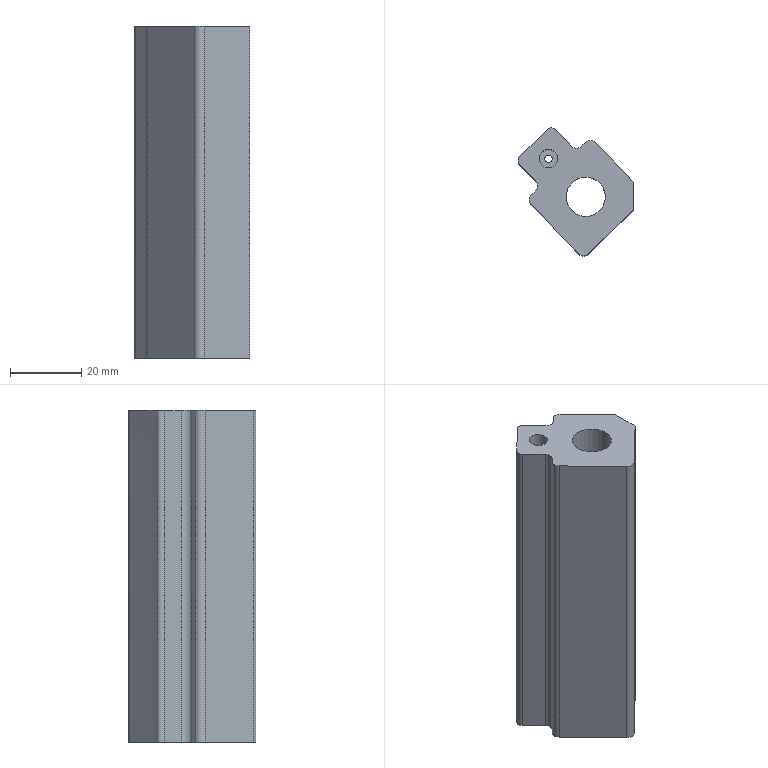Part | STEP file | gslz 2016.10.28-10_id2886_x_t | 1 solid | 24 faces | box 32.472 x 35.825 x 93 mm | volume 45038 mm3 | plane 12 | cylinder 11 | other 1 | commonest cylinder face diameters 4 x5 3 x2 2.1 x1 5.2 x1 11 x1 17 x1